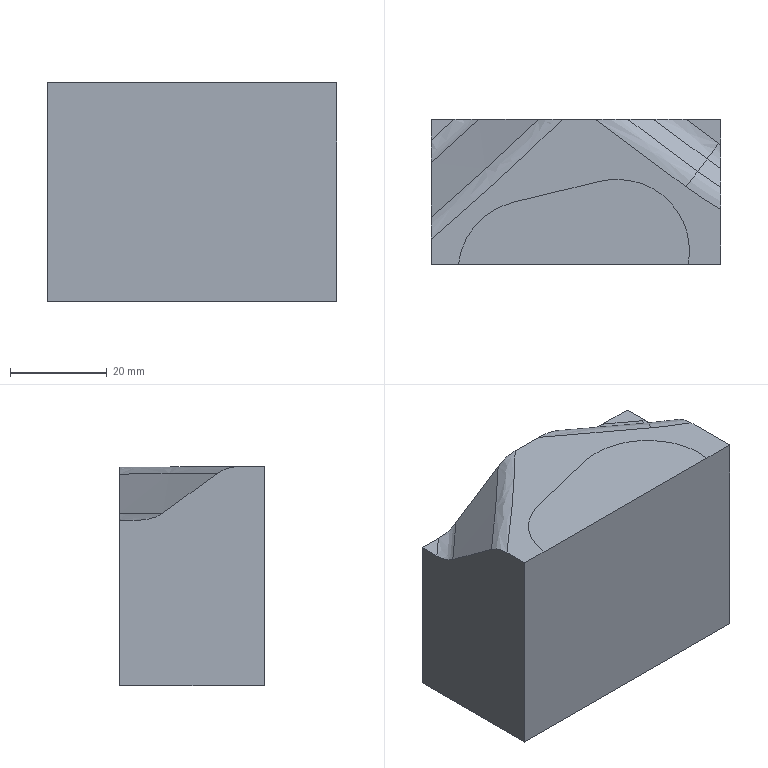Part | NX | features solid 2 | 1 solid | 18 faces | box 60 x 30 x 45.393 mm | volume 79393 mm3 | spline 13 | plane 5
STEP:
#1=CARTESIAN_POINT('',(-430.,-95.,60.393));
#2=VERTEX_POINT('',#1);
#3=CARTESIAN_POINT('',(-424.352,-95.,60.385));
#4=VERTEX_POINT('',#3);
#5=CARTESIAN_POINT('',(-429.926,-95.,60.393));
#6=DIRECTION('',(1.,0.,-0.001477));
#7=VECTOR('',#6,1000.);
#8=LINE('',#5,#7);
#9=EDGE_CURVE('',#2,#4,#8,.T.);
#10=ORIENTED_EDGE('',*,*,#9,.F.);
#11=CARTESIAN_POINT('',(-430.,-95.,15.));
#12=VERTEX_POINT('',#11);
#13=CARTESIAN_POINT('',(-430.,-95.,10.));
#14=DIRECTION('',(0.,0.,1.));
#15=VECTOR('',#14,1000.);
#16=LINE('',#13,#15);
#17=EDGE_CURVE('',#12,#2,#16,.T.);
#18=ORIENTED_EDGE('',*,*,#17,.F.);
#19=CARTESIAN_POINT('',(-370.,-95.,15.));
#20=VERTEX_POINT('',#19);
#21=CARTESIAN_POINT('',(-430.,-95.,15.));
#22=DIRECTION('',(1.,0.,0.));
#23=VECTOR('',#22,1000.);
#24=LINE('',#21,#23);
#25=EDGE_CURVE('',#12,#20,#24,.T.);
#26=ORIENTED_EDGE('',*,*,#25,.T.);
#27=CARTESIAN_POINT('',(-370.,-95.,60.305));
#28=VERTEX_POINT('',#27);
#29=CARTESIAN_POINT('',(-370.,-95.,10.));
#30=DIRECTION('',(0.,0.,1.));
#31=VECTOR('',#30,1000.);
#32=LINE('',#29,#31);
#33=EDGE_CURVE('',#20,#28,#32,.T.);
#34=ORIENTED_EDGE('',*,*,#33,.T.);
#35=CARTESIAN_POINT('',(-376.703,-95.,60.314));
#36=VERTEX_POINT('',#35);
#37=CARTESIAN_POINT('',(-429.926,-95.,60.393));
#38=DIRECTION('',(1.,0.,-0.001477));
#39=VECTOR('',#38,1000.);
#40=LINE('',#37,#39);
#41=EDGE_CURVE('',#36,#28,#40,.T.);
#42=ORIENTED_EDGE('',*,*,#41,.F.);
#43=CARTESIAN_POINT('',(-429.926,-95.,60.393));
#44=DIRECTION('',(1.,0.,-0.001477));
#45=VECTOR('',#44,1000.);
#46=LINE('',#43,#45);
#47=EDGE_CURVE('',#4,#36,#46,.T.);
#48=ORIENTED_EDGE('',*,*,#47,.F.);
#49=EDGE_LOOP('',(#10,#18,#26,#34,#42,#48));
#50=FACE_BOUND('',#49,.T.);
#51=CARTESIAN_POINT('',(-430.,-95.,10.));
#52=DIRECTION('',(0.,-1.,0.));
#53=DIRECTION('',(0.,0.,1.));
#54=AXIS2_PLACEMENT_3D('',#51,#52,#53);
#55=PLANE('',#54);
#56=ADVANCED_FACE('',(#50),#55,.T.);
#57=CARTESIAN_POINT('',(-425.27,-65.,49.259));
#58=VERTEX_POINT('',#57);
#59=CARTESIAN_POINT('',(-430.,-65.,49.276));
#60=VERTEX_POINT('',#59);
#61=CARTESIAN_POINT('',(-429.855,-65.,49.276));
#62=DIRECTION('',(1.,0.,-0.003698));
#63=VECTOR('',#62,1000.);
#64=LINE('',#61,#63);
#65=EDGE_CURVE('',#58,#60,#64,.F.);
#66=ORIENTED_EDGE('',*,*,#65,.F.);
#67=CARTESIAN_POINT('',(-420.138,-65.,50.648));
#68=VERTEX_POINT('',#67);
#69=CARTESIAN_POINT('',(-425.274,-65.,49.259));
#70=CARTESIAN_POINT('',(-423.471,-65.,49.252));
#71=CARTESIAN_POINT('',(-421.65,-65.,49.659));
#72=CARTESIAN_POINT('',(-420.138,-65.,50.648));
#73=B_SPLINE_CURVE_WITH_KNOTS('',3,(#69,#70,#71,#72),.UNSPECIFIED.,.F.,.F.,(4,4),(0.,0.005391),.UNSPECIFIED.);
#74=EDGE_CURVE('',#58,#68,#73,.T.);
#75=ORIENTED_EDGE('',*,*,#74,.T.);
#76=CARTESIAN_POINT('',(-407.783,-65.,58.79));
#77=VERTEX_POINT('',#76);
#78=CARTESIAN_POINT('',(-407.783,-65.,58.79));
#79=CARTESIAN_POINT('',(-411.892,-65.,56.061));
#80=CARTESIAN_POINT('',(-416.01,-65.,53.346));
#81=CARTESIAN_POINT('',(-420.138,-65.,50.648));
#82=B_SPLINE_CURVE_WITH_KNOTS('',3,(#78,#79,#80,#81),.UNSPECIFIED.,.F.,.F.,(4,4),(0.00008889,0.01488),.UNSPECIFIED.);
#83=EDGE_CURVE('',#77,#68,#82,.T.);
#84=ORIENTED_EDGE('',*,*,#83,.F.);
#85=CARTESIAN_POINT('',(-402.801,-65.,60.174));
#86=VERTEX_POINT('',#85);
#87=CARTESIAN_POINT('',(-407.783,-65.,58.79));
#88=CARTESIAN_POINT('',(-406.319,-65.,59.762));
#89=CARTESIAN_POINT('',(-404.555,-65.,60.177));
#90=CARTESIAN_POINT('',(-402.801,-65.,60.174));
#91=B_SPLINE_CURVE_WITH_KNOTS('',3,(#87,#88,#89,#90),.UNSPECIFIED.,.F.,.F.,(4,4),(0.,0.005252),.UNSPECIFIED.);
#92=EDGE_CURVE('',#77,#86,#91,.T.);
#93=ORIENTED_EDGE('',*,*,#92,.T.);
#94=CARTESIAN_POINT('',(-395.934,-65.,60.164));
#95=VERTEX_POINT('',#94);
#96=CARTESIAN_POINT('',(-429.926,-65.,60.214));
#97=DIRECTION('',(1.,0.,-0.001477));
#98=VECTOR('',#97,1000.);
#99=LINE('',#96,#98);
#100=EDGE_CURVE('',#95,#86,#99,.F.);
#101=ORIENTED_EDGE('',*,*,#100,.F.);
#102=CARTESIAN_POINT('',(-389.261,-65.,58.622));
#103=VERTEX_POINT('',#102);
#104=CARTESIAN_POINT('',(-395.934,-65.,60.164));
#105=CARTESIAN_POINT('',(-393.624,-65.,60.161));
#106=CARTESIAN_POINT('',(-391.295,-65.,59.722));
#107=CARTESIAN_POINT('',(-389.261,-65.,58.622));
#108=B_SPLINE_CURVE_WITH_KNOTS('',3,(#104,#105,#106,#107),.UNSPECIFIED.,.F.,.F.,(4,4),(0.,0.006914),.UNSPECIFIED.);
#109=EDGE_CURVE('',#95,#103,#108,.T.);
#110=ORIENTED_EDGE('',*,*,#109,.T.);
#111=CARTESIAN_POINT('',(-383.886,-65.,55.715));
#112=VERTEX_POINT('',#111);
#113=CARTESIAN_POINT('',(-400.43,-65.,64.664));
#114=DIRECTION('',(-0.8796,0.,0.4758));
#115=VECTOR('',#114,1000.);
#116=LINE('',#113,#115);
#117=EDGE_CURVE('',#103,#112,#116,.F.);
#118=ORIENTED_EDGE('',*,*,#117,.T.);
#119=CARTESIAN_POINT('',(-377.192,-65.,54.164));
#120=VERTEX_POINT('',#119);
#121=CARTESIAN_POINT('',(-377.192,-65.,54.164));
#122=CARTESIAN_POINT('',(-379.509,-65.,54.17));
#123=CARTESIAN_POINT('',(-381.845,-65.,54.611));
#124=CARTESIAN_POINT('',(-383.886,-65.,55.715));
#125=B_SPLINE_CURVE_WITH_KNOTS('',3,(#121,#122,#123,#124),.UNSPECIFIED.,.F.,.F.,(4,4),(0.000043,0.00698),.UNSPECIFIED.);
#126=EDGE_CURVE('',#120,#112,#125,.T.);
#127=ORIENTED_EDGE('',*,*,#126,.F.);
#128=CARTESIAN_POINT('',(-370.,-65.,54.145));
#129=VERTEX_POINT('',#128);
#130=CARTESIAN_POINT('',(-429.886,-65.,54.3));
#131=DIRECTION('',(1.,0.,-0.002576));
#132=VECTOR('',#131,1000.);
#133=LINE('',#130,#132);
#134=EDGE_CURVE('',#129,#120,#133,.F.);
#135=ORIENTED_EDGE('',*,*,#134,.F.);
#136=CARTESIAN_POINT('',(-370.,-65.,15.));
#137=VERTEX_POINT('',#136);
#138=CARTESIAN_POINT('',(-370.,-65.,10.));
#139=DIRECTION('',(0.,0.,1.));
#140=VECTOR('',#139,1000.);
#141=LINE('',#138,#140);
#142=EDGE_CURVE('',#137,#129,#141,.T.);
#143=ORIENTED_EDGE('',*,*,#142,.F.);
#144=CARTESIAN_POINT('',(-430.,-65.,15.));
#145=VERTEX_POINT('',#144);
#146=CARTESIAN_POINT('',(-430.,-65.,15.));
#147=DIRECTION('',(-1.,0.,0.));
#148=VECTOR('',#147,1000.);
#149=LINE('',#146,#148);
#150=EDGE_CURVE('',#145,#137,#149,.F.);
#151=ORIENTED_EDGE('',*,*,#150,.F.);
#152=CARTESIAN_POINT('',(-430.,-65.,10.));
#153=DIRECTION('',(0.,0.,1.));
#154=VECTOR('',#153,1000.);
#155=LINE('',#152,#154);
#156=EDGE_CURVE('',#145,#60,#155,.T.);
#157=ORIENTED_EDGE('',*,*,#156,.T.);
#158=EDGE_LOOP('',(#66,#75,#84,#93,#101,#110,#118,#127,#135,#143,#151,#157));
#159=FACE_BOUND('',#158,.T.);
#160=CARTESIAN_POINT('',(-430.,-65.,10.));
#161=DIRECTION('',(0.,-1.,0.));
#162=DIRECTION('',(0.,0.,1.));
#163=AXIS2_PLACEMENT_3D('',#160,#161,#162);
#164=PLANE('',#163);
#165=ADVANCED_FACE('',(#159),#164,.F.);
#166=CARTESIAN_POINT('',(-370.,-83.647,60.237));
#167=VERTEX_POINT('',#166);
#168=CARTESIAN_POINT('',(-370.,-64.701,60.124));
#169=DIRECTION('',(0.,-1.,0.005958));
#170=VECTOR('',#169,1000.);
#171=LINE('',#168,#170);
#172=EDGE_CURVE('',#28,#167,#171,.F.);
#173=ORIENTED_EDGE('',*,*,#172,.F.);
#174=ORIENTED_EDGE('',*,*,#33,.F.);
#175=CARTESIAN_POINT('',(-370.,-65.,15.));
#176=DIRECTION('',(0.,1.,0.));
#177=VECTOR('',#176,1000.);
#178=LINE('',#175,#177);
#179=EDGE_CURVE('',#137,#20,#178,.F.);
#180=ORIENTED_EDGE('',*,*,#179,.F.);
#181=ORIENTED_EDGE('',*,*,#142,.T.);
#182=CARTESIAN_POINT('',(-370.,-70.351,54.17));
#183=VERTEX_POINT('',#182);
#184=CARTESIAN_POINT('',(-370.,-64.798,54.145));
#185=DIRECTION('',(0.,-1.,0.004576));
#186=VECTOR('',#185,1000.);
#187=LINE('',#184,#186);
#188=EDGE_CURVE('',#183,#129,#187,.F.);
#189=ORIENTED_EDGE('',*,*,#188,.F.);
#190=CARTESIAN_POINT('',(-370.,-75.202,55.727));
#191=VERTEX_POINT('',#190);
#192=CARTESIAN_POINT('',(-370.,-75.202,55.726));
#193=CARTESIAN_POINT('',(-370.,-73.815,54.672));
#194=CARTESIAN_POINT('',(-370.,-72.09,54.178));
#195=CARTESIAN_POINT('',(-370.,-70.351,54.17));
#196=B_SPLINE_CURVE_WITH_KNOTS('',3,(#192,#193,#194,#195),.UNSPECIFIED.,.F.,.F.,(4,4),(0.,0.005159),.UNSPECIFIED.);
#197=EDGE_CURVE('',#191,#183,#196,.T.);
#198=ORIENTED_EDGE('',*,*,#197,.F.);
#199=CARTESIAN_POINT('',(-370.,-79.036,58.677));
#200=VERTEX_POINT('',#199);
#201=CARTESIAN_POINT('',(-370.,-75.203,55.727));
#202=CARTESIAN_POINT('',(-370.,-76.486,56.703));
#203=CARTESIAN_POINT('',(-370.,-77.764,57.687));
#204=CARTESIAN_POINT('',(-370.,-79.036,58.677));
#205=B_SPLINE_CURVE_WITH_KNOTS('',3,(#201,#202,#203,#204),.UNSPECIFIED.,.F.,.F.,(4,4),(0.00008367,0.004921),.UNSPECIFIED.);
#206=EDGE_CURVE('',#191,#200,#205,.T.);
#207=ORIENTED_EDGE('',*,*,#206,.T.);
#208=CARTESIAN_POINT('',(-370.,-83.646,60.237));
#209=CARTESIAN_POINT('',(-370.,-81.988,60.227));
#210=CARTESIAN_POINT('',(-370.,-80.346,59.696));
#211=CARTESIAN_POINT('',(-370.,-79.036,58.677));
#212=B_SPLINE_CURVE_WITH_KNOTS('',3,(#208,#209,#210,#211),.UNSPECIFIED.,.F.,.F.,(4,4),(0.,0.004923),.UNSPECIFIED.);
#213=EDGE_CURVE('',#167,#200,#212,.T.);
#214=ORIENTED_EDGE('',*,*,#213,.F.);
#215=EDGE_LOOP('',(#173,#174,#180,#181,#189,#198,#207,#214));
#216=FACE_BOUND('',#215,.T.);
#217=CARTESIAN_POINT('',(-370.,-65.,10.));
#218=DIRECTION('',(-1.,0.,0.));
#219=DIRECTION('',(0.,0.,1.));
#220=AXIS2_PLACEMENT_3D('',#217,#218,#219);
#221=PLANE('',#220);
#222=ADVANCED_FACE('',(#216),#221,.F.);
#223=CARTESIAN_POINT('',(-430.,-69.285,49.284));
#224=VERTEX_POINT('',#223);
#225=CARTESIAN_POINT('',(-430.,-73.938,50.7));
#226=VERTEX_POINT('',#225);
#227=CARTESIAN_POINT('',(-430.,-69.278,49.284));
#228=CARTESIAN_POINT('',(-430.,-70.934,49.287));
#229=CARTESIAN_POINT('',(-430.,-72.595,49.725));
#230=CARTESIAN_POINT('',(-430.,-73.938,50.7));
#231=B_SPLINE_CURVE_WITH_KNOTS('',3,(#227,#228,#229,#230),.UNSPECIFIED.,.F.,.F.,(4,4),(0.,0.004952),.UNSPECIFIED.);
#232=EDGE_CURVE('',#224,#226,#231,.T.);
#233=ORIENTED_EDGE('',*,*,#232,.F.);
#234=CARTESIAN_POINT('',(-430.,-64.931,49.276));
#235=DIRECTION('',(0.,-1.,0.00175));
#236=VECTOR('',#235,1000.);
#237=LINE('',#234,#236);
#238=EDGE_CURVE('',#224,#60,#237,.F.);
#239=ORIENTED_EDGE('',*,*,#238,.T.);
#240=ORIENTED_EDGE('',*,*,#156,.F.);
#241=CARTESIAN_POINT('',(-430.,-65.,15.));
#242=DIRECTION('',(0.,1.,0.));
#243=VECTOR('',#242,1000.);
#244=LINE('',#241,#243);
#245=EDGE_CURVE('',#145,#12,#244,.F.);
#246=ORIENTED_EDGE('',*,*,#245,.T.);
#247=ORIENTED_EDGE('',*,*,#17,.T.);
#248=CARTESIAN_POINT('',(-430.,-89.798,60.362));
#249=VERTEX_POINT('',#248);
#250=CARTESIAN_POINT('',(-430.,-64.701,60.213));
#251=DIRECTION('',(0.,-1.,0.005958));
#252=VECTOR('',#251,1000.);
#253=LINE('',#250,#252);
#254=EDGE_CURVE('',#2,#249,#253,.F.);
#255=ORIENTED_EDGE('',*,*,#254,.T.);
#256=CARTESIAN_POINT('',(-430.,-85.235,58.943));
#257=VERTEX_POINT('',#256);
#258=CARTESIAN_POINT('',(-430.,-85.235,58.943));
#259=CARTESIAN_POINT('',(-430.,-86.549,59.908));
#260=CARTESIAN_POINT('',(-430.,-88.17,60.352));
#261=CARTESIAN_POINT('',(-430.,-89.797,60.362));
#262=B_SPLINE_CURVE_WITH_KNOTS('',3,(#258,#259,#260,#261),.UNSPECIFIED.,.F.,.F.,(4,4),(0.,0.004839),.UNSPECIFIED.);
#263=EDGE_CURVE('',#257,#249,#262,.T.);
#264=ORIENTED_EDGE('',*,*,#263,.F.);
#265=CARTESIAN_POINT('',(-430.,-85.235,58.943));
#266=CARTESIAN_POINT('',(-430.,-81.476,56.185));
#267=CARTESIAN_POINT('',(-430.,-77.711,53.438));
#268=CARTESIAN_POINT('',(-430.,-73.938,50.7));
#269=B_SPLINE_CURVE_WITH_KNOTS('',3,(#265,#266,#267,#268),.UNSPECIFIED.,.F.,.F.,(4,4),(0.000084,0.01407),.UNSPECIFIED.);
#270=EDGE_CURVE('',#257,#226,#269,.T.);
#271=ORIENTED_EDGE('',*,*,#270,.T.);
#272=EDGE_LOOP('',(#233,#239,#240,#246,#247,#255,#264,#271));
#273=FACE_BOUND('',#272,.T.);
#274=CARTESIAN_POINT('',(-430.,-65.,10.));
#275=DIRECTION('',(-1.,0.,0.));
#276=DIRECTION('',(0.,0.,1.));
#277=AXIS2_PLACEMENT_3D('',#274,#275,#276);
#278=PLANE('',#277);
#279=ADVANCED_FACE('',(#273),#278,.T.);
#280=ORIENTED_EDGE('',*,*,#150,.T.);
#281=ORIENTED_EDGE('',*,*,#179,.T.);
#282=ORIENTED_EDGE('',*,*,#25,.F.);
#283=ORIENTED_EDGE('',*,*,#245,.F.);
#284=EDGE_LOOP('',(#280,#281,#282,#283));
#285=FACE_BOUND('',#284,.T.);
#286=CARTESIAN_POINT('',(-430.,-65.,15.));
#287=DIRECTION('',(0.,0.,-1.));
#288=DIRECTION('',(0.,-1.,0.));
#289=AXIS2_PLACEMENT_3D('',#286,#287,#288);
#290=PLANE('',#289);
#291=ADVANCED_FACE('',(#285),#290,.T.);
#292=ORIENTED_EDGE('',*,*,#47,.T.);
#293=CARTESIAN_POINT('',(-394.978,-77.819,60.239));
#294=VERTEX_POINT('',#293);
#295=CARTESIAN_POINT('',(-376.705,-94.999,60.314));
#296=CARTESIAN_POINT('',(-376.275,-92.541,60.299));
#297=CARTESIAN_POINT('',(-376.637,-87.429,60.269));
#298=CARTESIAN_POINT('',(-380.148,-82.049,60.242));
#299=CARTESIAN_POINT('',(-384.224,-79.074,60.231));
#300=CARTESIAN_POINT('',(-387.107,-77.972,60.228));
#301=CARTESIAN_POINT('',(-389.571,-77.528,60.229));
#302=CARTESIAN_POINT('',(-391.094,-77.444,60.231));
#303=CARTESIAN_POINT('',(-392.189,-77.471,60.233));
#304=CARTESIAN_POINT('',(-392.865,-77.517,60.234));
#305=CARTESIAN_POINT('',(-393.655,-77.591,60.236));
#306=CARTESIAN_POINT('',(-394.358,-77.698,60.237));
#307=CARTESIAN_POINT('',(-394.979,-77.816,60.239));
#308=B_SPLINE_CURVE_WITH_KNOTS('',3,(#295,#296,#297,#298,#299,#300,#301,#302,#303,#304,#305,#306,#307),.UNSPECIFIED.,.F.,.F.,(4,1,1,1,1,1,1,1,1,1,4),(0.6328,0.6897,0.7467,0.7751,0.8036,0.8178,0.8321,0.8392,0.8427,0.8463,0.8605),.UNSPECIFIED.);
#309=EDGE_CURVE('',#36,#294,#308,.T.);
#310=ORIENTED_EDGE('',*,*,#309,.T.);
#311=CARTESIAN_POINT('',(-412.965,-82.147,60.291));
#312=VERTEX_POINT('',#311);
#313=CARTESIAN_POINT('',(-394.979,-77.816,60.239));
#314=CARTESIAN_POINT('',(-395.358,-77.888,60.24));
#315=CARTESIAN_POINT('',(-395.944,-78.012,60.242));
#316=CARTESIAN_POINT('',(-396.713,-78.195,60.244));
#317=CARTESIAN_POINT('',(-397.111,-78.296,60.245));
#318=CARTESIAN_POINT('',(-397.49,-78.391,60.246));
#319=CARTESIAN_POINT('',(-398.186,-78.566,60.248));
#320=CARTESIAN_POINT('',(-399.446,-78.879,60.252));
#321=CARTESIAN_POINT('',(-401.216,-79.314,60.257));
#322=CARTESIAN_POINT('',(-403.217,-79.801,60.263));
#323=CARTESIAN_POINT('',(-404.724,-80.165,60.267));
#324=CARTESIAN_POINT('',(-405.531,-80.36,60.27));
#325=CARTESIAN_POINT('',(-405.963,-80.464,60.271));
#326=CARTESIAN_POINT('',(-406.545,-80.604,60.273));
#327=CARTESIAN_POINT('',(-407.327,-80.792,60.275));
#328=CARTESIAN_POINT('',(-408.437,-81.059,60.278));
#329=CARTESIAN_POINT('',(-410.177,-81.477,60.283));
#330=CARTESIAN_POINT('',(-411.996,-81.914,60.289));
#331=CARTESIAN_POINT('',(-412.758,-82.098,60.291));
#332=CARTESIAN_POINT('',(-412.965,-82.147,60.291));
#333=B_SPLINE_CURVE_WITH_KNOTS('',3,(#313,#314,#315,#316,#317,#318,#319,#320,#321,#322,#323,#324,#325,#326,#327,#328,#329,#330,#331,#332),.UNSPECIFIED.,.F.,.F.,(4,1,1,1,1,1,1,1,1,1,1,1,1,1,1,1,1,4),(0.8605,0.8693,0.8736,0.8758,0.878,0.8867,0.8954,0.9128,0.9303,0.939,0.9433,0.9455,0.9477,0.9521,0.9564,0.9651,0.9826,1.),.UNSPECIFIED.);
#334=EDGE_CURVE('',#294,#312,#333,.T.);
#335=ORIENTED_EDGE('',*,*,#334,.T.);
#336=CARTESIAN_POINT('',(-412.965,-82.147,60.291));
#337=CARTESIAN_POINT('',(-415.91,-82.856,60.3));
#338=CARTESIAN_POINT('',(-420.051,-85.39,60.321));
#339=CARTESIAN_POINT('',(-423.351,-90.457,60.356));
#340=CARTESIAN_POINT('',(-424.171,-93.491,60.376));
#341=CARTESIAN_POINT('',(-424.35,-95.,60.385));
#342=B_SPLINE_CURVE_WITH_KNOTS('',3,(#336,#337,#338,#339,#340,#341),.UNSPECIFIED.,.F.,.F.,(4,1,1,4),(0.,0.06962,0.1044,0.1392),.UNSPECIFIED.);
#343=EDGE_CURVE('',#312,#4,#342,.T.);
#344=ORIENTED_EDGE('',*,*,#343,.T.);
#345=EDGE_LOOP('',(#292,#310,#335,#344));
#346=FACE_BOUND('',#345,.T.);
#347=CARTESIAN_POINT('',(-424.637,-95.106,60.386));
#348=CARTESIAN_POINT('',(-376.173,-95.106,60.314));
#349=CARTESIAN_POINT('',(-424.637,-77.33,60.28));
#350=CARTESIAN_POINT('',(-376.173,-77.33,60.208));
#351=B_SPLINE_SURFACE_WITH_KNOTS('',1,1,((#347,#348),(#349,#350)),.PLANE_SURF.,.F.,.F.,.F.,(2,2),(2,2),(0.7159,0.8657),(0.2377,0.4034),.PIECEWISE_BEZIER_KNOTS.);
#352=ADVANCED_FACE('',(#346),#351,.F.);
#353=CARTESIAN_POINT('',(-377.227,-78.986,60.22));
#354=VERTEX_POINT('',#353);
#355=CARTESIAN_POINT('',(-377.227,-78.986,60.22));
#356=CARTESIAN_POINT('',(-383.463,-74.324,60.201));
#357=CARTESIAN_POINT('',(-389.698,-69.662,60.183));
#358=CARTESIAN_POINT('',(-395.934,-65.,60.164));
#359=B_SPLINE_CURVE_WITH_KNOTS('',3,(#355,#356,#357,#358),.UNSPECIFIED.,.F.,.F.,(4,4),(0.,0.8279),.UNSPECIFIED.);
#360=EDGE_CURVE('',#95,#354,#359,.F.);
#361=ORIENTED_EDGE('',*,*,#360,.T.);
#362=CARTESIAN_POINT('',(-374.832,-75.788,58.665));
#363=VERTEX_POINT('',#362);
#364=CARTESIAN_POINT('',(-374.832,-75.788,58.665));
#365=CARTESIAN_POINT('',(-375.468,-76.635,59.625));
#366=CARTESIAN_POINT('',(-376.372,-77.842,60.212));
#367=CARTESIAN_POINT('',(-377.227,-78.986,60.22));
#368=B_SPLINE_CURVE_WITH_KNOTS('',3,(#364,#365,#366,#367),.UNSPECIFIED.,.F.,.F.,(4,4),(0.,1.),.UNSPECIFIED.);
#369=EDGE_CURVE('',#354,#363,#368,.F.);
#370=ORIENTED_EDGE('',*,*,#369,.T.);
#371=CARTESIAN_POINT('',(-389.261,-65.,58.622));
#372=CARTESIAN_POINT('',(-384.451,-68.596,58.637));
#373=CARTESIAN_POINT('',(-379.641,-72.192,58.651));
#374=CARTESIAN_POINT('',(-374.832,-75.788,58.665));
#375=B_SPLINE_CURVE_WITH_KNOTS('',3,(#371,#372,#373,#374),.UNSPECIFIED.,.F.,.F.,(4,4),(0.3652,1.),.UNSPECIFIED.);
#376=EDGE_CURVE('',#103,#363,#375,.T.);
#377=ORIENTED_EDGE('',*,*,#376,.F.);
#378=ORIENTED_EDGE('',*,*,#109,.F.);
#379=EDGE_LOOP('',(#361,#370,#377,#378));
#380=FACE_BOUND('',#379,.T.);
#381=CARTESIAN_POINT('',(-374.832,-75.788,58.665));
#382=CARTESIAN_POINT('',(-393.65,-61.718,58.609));
#383=CARTESIAN_POINT('',(-375.497,-76.674,59.669));
#384=CARTESIAN_POINT('',(-394.315,-62.604,59.613));
#385=CARTESIAN_POINT('',(-376.332,-77.789,60.211));
#386=CARTESIAN_POINT('',(-395.151,-63.719,60.155));
#387=CARTESIAN_POINT('',(-377.227,-78.986,60.22));
#388=CARTESIAN_POINT('',(-396.046,-64.916,60.164));
#389=(BOUNDED_SURFACE()B_SPLINE_SURFACE(3,1,((#381,#382),(#383,#384),(#385,#386),(#387,#388)),.CYLINDRICAL_SURF.,.F.,.F.,.F.)B_SPLINE_SURFACE_WITH_KNOTS((4,4),(2,2),(0.006098,1.),(0.,0.823),.PIECEWISE_BEZIER_KNOTS.)GEOMETRIC_REPRESENTATION_ITEM()RATIONAL_B_SPLINE_SURFACE(((0.9992,0.9992),(0.9555,0.9555),(0.9557,0.9557),(1.,1.)))REPRESENTATION_ITEM('')SURFACE());
#390=ADVANCED_FACE('',(#380),#389,.F.);
#391=ORIENTED_EDGE('',*,*,#376,.T.);
#392=CARTESIAN_POINT('',(-372.883,-73.194,55.724));
#393=VERTEX_POINT('',#392);
#394=CARTESIAN_POINT('',(-374.832,-75.788,58.665));
#395=CARTESIAN_POINT('',(-374.182,-74.924,57.685));
#396=CARTESIAN_POINT('',(-373.533,-74.059,56.705));
#397=CARTESIAN_POINT('',(-372.883,-73.194,55.724));
#398=B_SPLINE_CURVE_WITH_KNOTS('',3,(#394,#395,#396,#397),.UNSPECIFIED.,.F.,.F.,(4,4),(0.,1.),.UNSPECIFIED.);
#399=EDGE_CURVE('',#363,#393,#398,.T.);
#400=ORIENTED_EDGE('',*,*,#399,.T.);
#401=CARTESIAN_POINT('',(-372.883,-73.194,55.724));
#402=CARTESIAN_POINT('',(-376.551,-70.463,55.721));
#403=CARTESIAN_POINT('',(-380.219,-67.731,55.718));
#404=CARTESIAN_POINT('',(-383.886,-65.,55.715));
#405=B_SPLINE_CURVE_WITH_KNOTS('',3,(#401,#402,#403,#404),.UNSPECIFIED.,.F.,.F.,(4,4),(0.,0.4436),.UNSPECIFIED.);
#406=EDGE_CURVE('',#393,#112,#405,.T.);
#407=ORIENTED_EDGE('',*,*,#406,.T.);
#408=ORIENTED_EDGE('',*,*,#117,.F.);
#409=EDGE_LOOP('',(#391,#400,#407,#408));
#410=FACE_BOUND('',#409,.T.);
#411=CARTESIAN_POINT('',(-389.359,-63.541,57.614));
#412=CARTESIAN_POINT('',(-372.785,-67.806,51.751));
#413=CARTESIAN_POINT('',(-389.359,-72.101,63.841));
#414=CARTESIAN_POINT('',(-372.785,-76.366,57.978));
#415=B_SPLINE_SURFACE_WITH_KNOTS('',1,1,((#411,#412),(#413,#414)),.PLANE_SURF.,.F.,.F.,.F.,(2,2),(2,2),(0.4403,0.9974),(0.3377,0.998),.PIECEWISE_BEZIER_KNOTS.);
#416=ADVANCED_FACE('',(#410),#415,.T.);
#417=ORIENTED_EDGE('',*,*,#126,.T.);
#418=ORIENTED_EDGE('',*,*,#406,.F.);
#419=CARTESIAN_POINT('',(-370.494,-69.988,54.17));
#420=VERTEX_POINT('',#419);
#421=CARTESIAN_POINT('',(-372.883,-73.194,55.724));
#422=CARTESIAN_POINT('',(-372.25,-72.345,54.764));
#423=CARTESIAN_POINT('',(-371.349,-71.135,54.177));
#424=CARTESIAN_POINT('',(-370.494,-69.988,54.17));
#425=B_SPLINE_CURVE_WITH_KNOTS('',3,(#421,#422,#423,#424),.UNSPECIFIED.,.F.,.F.,(4,4),(0.,1.),.UNSPECIFIED.);
#426=EDGE_CURVE('',#393,#420,#425,.T.);
#427=ORIENTED_EDGE('',*,*,#426,.T.);
#428=CARTESIAN_POINT('',(-370.494,-69.988,54.17));
#429=CARTESIAN_POINT('',(-372.727,-68.325,54.168));
#430=CARTESIAN_POINT('',(-374.959,-66.663,54.166));
#431=CARTESIAN_POINT('',(-377.192,-65.,54.164));
#432=B_SPLINE_CURVE_WITH_KNOTS('',3,(#428,#429,#430,#431),.UNSPECIFIED.,.F.,.F.,(4,4),(0.,0.2545),.UNSPECIFIED.);
#433=EDGE_CURVE('',#420,#120,#432,.T.);
#434=ORIENTED_EDGE('',*,*,#433,.T.);
#435=EDGE_LOOP('',(#417,#418,#427,#434));
#436=FACE_BOUND('',#435,.T.);
#437=CARTESIAN_POINT('',(-372.883,-73.194,55.724));
#438=CARTESIAN_POINT('',(-383.952,-64.951,55.715));
#439=CARTESIAN_POINT('',(-372.221,-72.306,54.72));
#440=CARTESIAN_POINT('',(-383.29,-64.062,54.71));
#441=CARTESIAN_POINT('',(-371.388,-71.188,54.177));
#442=CARTESIAN_POINT('',(-382.457,-62.944,54.168));
#443=CARTESIAN_POINT('',(-370.494,-69.988,54.17));
#444=CARTESIAN_POINT('',(-381.563,-61.744,54.16));
#445=(BOUNDED_SURFACE()B_SPLINE_SURFACE(3,1,((#437,#438),(#439,#440),(#441,#442),(#443,#444)),.CYLINDRICAL_SURF.,.F.,.F.,.F.)B_SPLINE_SURFACE_WITH_KNOTS((4,4),(2,2),(0.,0.9939),(0.,0.4146),.PIECEWISE_BEZIER_KNOTS.)GEOMETRIC_REPRESENTATION_ITEM()RATIONAL_B_SPLINE_SURFACE(((1.,1.),(0.9557,0.9557),(0.9554,0.9554),(0.9992,0.9992)))REPRESENTATION_ITEM('')SURFACE());
#446=ADVANCED_FACE('',(#436),#445,.T.);
#447=ORIENTED_EDGE('',*,*,#213,.T.);
#448=CARTESIAN_POINT('',(-374.832,-75.788,58.665));
#449=CARTESIAN_POINT('',(-373.285,-76.945,58.67));
#450=CARTESIAN_POINT('',(-371.671,-78.031,58.674));
#451=CARTESIAN_POINT('',(-370.,-79.036,58.677));
#452=B_SPLINE_CURVE_WITH_KNOTS('',3,(#448,#449,#450,#451),.UNSPECIFIED.,.F.,.F.,(4,4),(0.,0.2094),.UNSPECIFIED.);
#453=EDGE_CURVE('',#363,#200,#452,.T.);
#454=ORIENTED_EDGE('',*,*,#453,.F.);
#455=ORIENTED_EDGE('',*,*,#369,.F.);
#456=CARTESIAN_POINT('',(-370.,-83.647,60.237));
#457=CARTESIAN_POINT('',(-372.526,-82.256,60.232));
#458=CARTESIAN_POINT('',(-374.945,-80.693,60.227));
#459=CARTESIAN_POINT('',(-377.227,-78.986,60.22));
#460=B_SPLINE_CURVE_WITH_KNOTS('',3,(#456,#457,#458,#459),.UNSPECIFIED.,.F.,.F.,(4,4),(0.7109,1.),.UNSPECIFIED.);
#461=EDGE_CURVE('',#354,#167,#460,.F.);
#462=ORIENTED_EDGE('',*,*,#461,.T.);
#463=EDGE_LOOP('',(#447,#454,#455,#462));
#464=FACE_BOUND('',#463,.T.);
#465=CARTESIAN_POINT('',(-368.028,-80.171,58.681));
#466=CARTESIAN_POINT('',(-370.4,-78.867,58.677));
#467=CARTESIAN_POINT('',(-372.672,-77.403,58.672));
#468=CARTESIAN_POINT('',(-374.832,-75.788,58.665));
#469=CARTESIAN_POINT('',(-368.562,-81.141,59.686));
#470=CARTESIAN_POINT('',(-370.981,-79.812,59.681));
#471=CARTESIAN_POINT('',(-373.295,-78.32,59.676));
#472=CARTESIAN_POINT('',(-375.497,-76.674,59.669));
#473=CARTESIAN_POINT('',(-369.234,-82.362,60.228));
#474=CARTESIAN_POINT('',(-371.709,-81.001,60.224));
#475=CARTESIAN_POINT('',(-374.079,-79.474,60.218));
#476=CARTESIAN_POINT('',(-376.332,-77.789,60.211));
#477=CARTESIAN_POINT('',(-369.954,-83.672,60.237));
#478=CARTESIAN_POINT('',(-372.491,-82.278,60.232));
#479=CARTESIAN_POINT('',(-374.919,-80.713,60.227));
#480=CARTESIAN_POINT('',(-377.227,-78.986,60.22));
#481=(BOUNDED_SURFACE()B_SPLINE_SURFACE(3,3,((#465,#466,#467,#468),(#469,#470,#471,#472),(#473,#474,#475,#476),(#477,#478,#479,#480)),.TOROIDAL_SURF.,.F.,.F.,.F.)B_SPLINE_SURFACE_WITH_KNOTS((4,4),(4,4),(0.,1.),(0.7092,1.),.PIECEWISE_BEZIER_KNOTS.)GEOMETRIC_REPRESENTATION_ITEM()RATIONAL_B_SPLINE_SURFACE(((0.9881,0.9905,0.9944,1.),(0.9446,0.9469,0.9507,0.956),(0.9446,0.9469,0.9507,0.956),(0.9881,0.9905,0.9944,1.)))REPRESENTATION_ITEM('')SURFACE());
#482=ADVANCED_FACE('',(#464),#481,.F.);
#483=ORIENTED_EDGE('',*,*,#134,.T.);
#484=ORIENTED_EDGE('',*,*,#433,.F.);
#485=CARTESIAN_POINT('',(-370.,-70.351,54.17));
#486=CARTESIAN_POINT('',(-370.165,-70.231,54.17));
#487=CARTESIAN_POINT('',(-370.33,-70.11,54.17));
#488=CARTESIAN_POINT('',(-370.494,-69.988,54.17));
#489=B_SPLINE_CURVE_WITH_KNOTS('',3,(#485,#486,#487,#488),.UNSPECIFIED.,.F.,.F.,(4,4),(0.975,1.),.UNSPECIFIED.);
#490=EDGE_CURVE('',#183,#420,#489,.T.);
#491=ORIENTED_EDGE('',*,*,#490,.F.);
#492=ORIENTED_EDGE('',*,*,#188,.T.);
#493=EDGE_LOOP('',(#483,#484,#491,#492));
#494=FACE_BOUND('',#493,.T.);
#495=CARTESIAN_POINT('',(-377.235,-70.384,54.189));
#496=CARTESIAN_POINT('',(-370.,-70.384,54.17));
#497=CARTESIAN_POINT('',(-377.235,-64.968,54.164));
#498=CARTESIAN_POINT('',(-370.,-64.968,54.145));
#499=B_SPLINE_SURFACE_WITH_KNOTS('',1,1,((#495,#496),(#497,#498)),.PLANE_SURF.,.F.,.F.,.F.,(2,2),(2,2),(0.472,0.5315),(0.1322,0.1788),.PIECEWISE_BEZIER_KNOTS.);
#500=ADVANCED_FACE('',(#494),#499,.F.);
#501=CARTESIAN_POINT('',(-370.,-75.202,55.727));
#502=CARTESIAN_POINT('',(-370.985,-74.562,55.726));
#503=CARTESIAN_POINT('',(-371.947,-73.892,55.725));
#504=CARTESIAN_POINT('',(-372.883,-73.194,55.724));
#505=B_SPLINE_CURVE_WITH_KNOTS('',3,(#501,#502,#503,#504),.UNSPECIFIED.,.F.,.F.,(4,4),(0.8659,1.),.UNSPECIFIED.);
#506=EDGE_CURVE('',#191,#393,#505,.T.);
#507=ORIENTED_EDGE('',*,*,#506,.T.);
#508=ORIENTED_EDGE('',*,*,#399,.F.);
#509=ORIENTED_EDGE('',*,*,#453,.T.);
#510=ORIENTED_EDGE('',*,*,#206,.F.);
#511=EDGE_LOOP('',(#507,#508,#509,#510));
#512=FACE_BOUND('',#511,.T.);
#513=CARTESIAN_POINT('',(-369.97,-79.055,58.677));
#514=CARTESIAN_POINT('',(-371.657,-78.04,58.674));
#515=CARTESIAN_POINT('',(-373.288,-76.944,58.67));
#516=CARTESIAN_POINT('',(-374.859,-75.768,58.665));
#517=CARTESIAN_POINT('',(-368.282,-76.256,55.713));
#518=CARTESIAN_POINT('',(-369.874,-75.299,55.71));
#519=CARTESIAN_POINT('',(-371.412,-74.264,55.706));
#520=CARTESIAN_POINT('',(-372.895,-73.155,55.701));
#521=(BOUNDED_SURFACE()B_SPLINE_SURFACE(1,3,((#513,#514,#515,#516),(#517,#518,#519,#520)),.CONICAL_SURF.,.F.,.F.,.F.)B_SPLINE_SURFACE_WITH_KNOTS((2,2),(4,4),(0.09091,0.99),(0.7859,0.9953),.PIECEWISE_BEZIER_KNOTS.)GEOMETRIC_REPRESENTATION_ITEM()RATIONAL_B_SPLINE_SURFACE(((0.9901,0.9924,0.9956,0.9997),(0.9901,0.9924,0.9956,0.9997)))REPRESENTATION_ITEM('')SURFACE());
#522=ADVANCED_FACE('',(#512),#521,.T.);
#523=ORIENTED_EDGE('',*,*,#197,.T.);
#524=ORIENTED_EDGE('',*,*,#490,.T.);
#525=ORIENTED_EDGE('',*,*,#426,.F.);
#526=ORIENTED_EDGE('',*,*,#506,.F.);
#527=EDGE_LOOP('',(#523,#524,#525,#526));
#528=FACE_BOUND('',#527,.T.);
#529=CARTESIAN_POINT('',(-370.494,-69.988,54.17));
#530=CARTESIAN_POINT('',(-371.018,-70.692,54.174));
#531=CARTESIAN_POINT('',(-371.542,-71.395,54.339));
#532=CARTESIAN_POINT('',(-372.042,-72.066,54.664));
#533=CARTESIAN_POINT('',(-372.495,-72.673,55.135));
#534=CARTESIAN_POINT('',(-372.883,-73.194,55.724));
#535=CARTESIAN_POINT('',(-369.969,-70.379,54.17));
#536=CARTESIAN_POINT('',(-370.484,-71.09,54.175));
#537=CARTESIAN_POINT('',(-370.998,-71.8,54.34));
#538=CARTESIAN_POINT('',(-371.489,-72.477,54.665));
#539=CARTESIAN_POINT('',(-371.934,-73.091,55.135));
#540=CARTESIAN_POINT('',(-372.316,-73.617,55.725));
#541=CARTESIAN_POINT('',(-369.437,-70.762,54.17));
#542=CARTESIAN_POINT('',(-369.942,-71.48,54.175));
#543=CARTESIAN_POINT('',(-370.448,-72.196,54.34));
#544=CARTESIAN_POINT('',(-370.93,-72.88,54.665));
#545=CARTESIAN_POINT('',(-371.367,-73.499,55.136));
#546=CARTESIAN_POINT('',(-371.742,-74.03,55.725));
#547=CARTESIAN_POINT('',(-368.898,-71.137,54.171));
#548=CARTESIAN_POINT('',(-369.395,-71.861,54.175));
#549=CARTESIAN_POINT('',(-369.891,-72.583,54.34));
#550=CARTESIAN_POINT('',(-370.365,-73.273,54.666));
#551=CARTESIAN_POINT('',(-370.794,-73.898,55.136));
#552=CARTESIAN_POINT('',(-371.162,-74.434,55.726));
#553=CARTESIAN_POINT('',(-368.354,-71.503,54.171));
#554=CARTESIAN_POINT('',(-368.842,-72.232,54.176));
#555=CARTESIAN_POINT('',(-369.329,-72.962,54.341));
#556=CARTESIAN_POINT('',(-369.793,-73.658,54.666));
#557=CARTESIAN_POINT('',(-370.214,-74.288,55.137));
#558=CARTESIAN_POINT('',(-370.575,-74.829,55.726));
#559=CARTESIAN_POINT('',(-367.805,-71.859,54.171));
#560=CARTESIAN_POINT('',(-368.282,-72.595,54.176));
#561=CARTESIAN_POINT('',(-368.76,-73.331,54.341));
#562=CARTESIAN_POINT('',(-369.215,-74.033,54.666));
#563=CARTESIAN_POINT('',(-369.628,-74.668,55.137));
#564=CARTESIAN_POINT('',(-369.982,-75.214,55.726));
#565=B_SPLINE_SURFACE_WITH_KNOTS('',5,5,((#529,#530,#531,#532,#533,#534),(#535,#536,#537,#538,#539,#540),(#541,#542,#543,#544,#545,#546),(#547,#548,#549,#550,#551,#552),(#553,#554,#555,#556,#557,#558),(#559,#560,#561,#562,#563,#564)),.UNSPECIFIED.,.F.,.F.,.F.,(6,6),(6,6),(0.,0.1341),(0.,1.),.PIECEWISE_BEZIER_KNOTS.);
#566=ADVANCED_FACE('',(#528),#565,.F.);
#567=ORIENTED_EDGE('',*,*,#65,.T.);
#568=ORIENTED_EDGE('',*,*,#238,.F.);
#569=CARTESIAN_POINT('',(-425.262,-65.004,49.259));
#570=CARTESIAN_POINT('',(-426.832,-66.44,49.267));
#571=CARTESIAN_POINT('',(-428.411,-67.868,49.275));
#572=CARTESIAN_POINT('',(-429.997,-69.288,49.284));
#573=B_SPLINE_CURVE_WITH_KNOTS('',3,(#569,#570,#571,#572),.UNSPECIFIED.,.F.,.F.,(4,4),(0.6554,0.7018),.UNSPECIFIED.);
#574=EDGE_CURVE('',#58,#224,#573,.T.);
#575=ORIENTED_EDGE('',*,*,#574,.F.);
#576=EDGE_LOOP('',(#567,#568,#575));
#577=FACE_BOUND('',#576,.T.);
#578=CARTESIAN_POINT('',(-430.,-69.317,49.284));
#579=CARTESIAN_POINT('',(-425.229,-69.317,49.266));
#580=CARTESIAN_POINT('',(-430.,-64.974,49.276));
#581=CARTESIAN_POINT('',(-425.229,-64.974,49.259));
#582=B_SPLINE_SURFACE_WITH_KNOTS('',1,1,((#578,#579),(#580,#581)),.PLANE_SURF.,.F.,.F.,.F.,(2,2),(2,2),(0.059,0.06724),(0.1423,0.1552),.PIECEWISE_BEZIER_KNOTS.);
#583=ADVANCED_FACE('',(#577),#582,.F.);
#584=ORIENTED_EDGE('',*,*,#574,.T.);
#585=ORIENTED_EDGE('',*,*,#232,.T.);
#586=CARTESIAN_POINT('',(-430.,-73.938,50.7));
#587=CARTESIAN_POINT('',(-426.679,-70.996,50.682));
#588=CARTESIAN_POINT('',(-423.392,-68.016,50.665));
#589=CARTESIAN_POINT('',(-420.138,-65.,50.648));
#590=B_SPLINE_CURVE_WITH_KNOTS('',3,(#586,#587,#588,#589),.UNSPECIFIED.,.F.,.F.,(4,4),(0.2762,0.3722),.UNSPECIFIED.);
#591=EDGE_CURVE('',#226,#68,#590,.T.);
#592=ORIENTED_EDGE('',*,*,#591,.T.);
#593=ORIENTED_EDGE('',*,*,#74,.F.);
#594=EDGE_LOOP('',(#584,#585,#592,#593));
#595=FACE_BOUND('',#594,.T.);
#596=CARTESIAN_POINT('',(-422.449,-62.398,49.244));
#597=CARTESIAN_POINT('',(-421.926,-62.962,49.243));
#598=CARTESIAN_POINT('',(-421.403,-63.526,49.39));
#599=CARTESIAN_POINT('',(-420.904,-64.061,49.685));
#600=CARTESIAN_POINT('',(-420.457,-64.541,50.113));
#601=CARTESIAN_POINT('',(-420.079,-64.946,50.647));
#602=CARTESIAN_POINT('',(-424.413,-64.219,49.254));
#603=CARTESIAN_POINT('',(-423.893,-64.785,49.253));
#604=CARTESIAN_POINT('',(-423.372,-65.351,49.4));
#605=CARTESIAN_POINT('',(-422.876,-65.889,49.695));
#606=CARTESIAN_POINT('',(-422.431,-66.371,50.123));
#607=CARTESIAN_POINT('',(-422.055,-66.777,50.658));
#608=CARTESIAN_POINT('',(-426.387,-66.028,49.265));
#609=CARTESIAN_POINT('',(-425.87,-66.597,49.264));
#610=CARTESIAN_POINT('',(-425.351,-67.166,49.411));
#611=CARTESIAN_POINT('',(-424.858,-67.706,49.706));
#612=CARTESIAN_POINT('',(-424.415,-68.19,50.134));
#613=CARTESIAN_POINT('',(-424.041,-68.598,50.668));
#614=CARTESIAN_POINT('',(-428.372,-67.827,49.275));
#615=CARTESIAN_POINT('',(-427.857,-68.398,49.274));
#616=CARTESIAN_POINT('',(-427.341,-68.969,49.421));
#617=CARTESIAN_POINT('',(-426.85,-69.512,49.716));
#618=CARTESIAN_POINT('',(-426.409,-69.998,50.145));
#619=CARTESIAN_POINT('',(-426.037,-70.407,50.679));
#620=CARTESIAN_POINT('',(-430.367,-69.614,49.286));
#621=CARTESIAN_POINT('',(-429.854,-70.188,49.285));
#622=CARTESIAN_POINT('',(-429.341,-70.761,49.432));
#623=CARTESIAN_POINT('',(-428.852,-71.306,49.727));
#624=CARTESIAN_POINT('',(-428.414,-71.794,50.155));
#625=CARTESIAN_POINT('',(-428.043,-72.205,50.69));
#626=CARTESIAN_POINT('',(-432.371,-71.39,49.296));
#627=CARTESIAN_POINT('',(-431.861,-71.966,49.295));
#628=CARTESIAN_POINT('',(-431.351,-72.542,49.442));
#629=CARTESIAN_POINT('',(-430.865,-73.089,49.738));
#630=CARTESIAN_POINT('',(-430.428,-73.579,50.166));
#631=CARTESIAN_POINT('',(-430.06,-73.991,50.7));
#632=B_SPLINE_SURFACE_WITH_KNOTS('',5,5,((#596,#597,#598,#599,#600,#601),(#602,#603,#604,#605,#606,#607),(#608,#609,#610,#611,#612,#613),(#614,#615,#616,#617,#618,#619),(#620,#621,#622,#623,#624,#625),(#626,#627,#628,#629,#630,#631)),.UNSPECIFIED.,.F.,.F.,.F.,(6,6),(6,6),(0.6272,0.7244),(0.,1.),.PIECEWISE_BEZIER_KNOTS.);
#633=ADVANCED_FACE('',(#595),#632,.T.);
#634=ORIENTED_EDGE('',*,*,#83,.T.);
#635=ORIENTED_EDGE('',*,*,#591,.F.);
#636=ORIENTED_EDGE('',*,*,#270,.F.);
#637=CARTESIAN_POINT('',(-407.783,-65.,58.79));
#638=CARTESIAN_POINT('',(-415.021,-71.931,58.842));
#639=CARTESIAN_POINT('',(-422.431,-78.68,58.893));
#640=CARTESIAN_POINT('',(-430.,-85.235,58.943));
#641=B_SPLINE_CURVE_WITH_KNOTS('',3,(#637,#638,#639,#640),.UNSPECIFIED.,.F.,.F.,(4,4),(0.1007,0.4936),.UNSPECIFIED.);
#642=EDGE_CURVE('',#77,#257,#641,.T.);
#643=ORIENTED_EDGE('',*,*,#642,.F.);
#644=EDGE_LOOP('',(#634,#635,#636,#643));
#645=FACE_BOUND('',#644,.T.);
#646=CARTESIAN_POINT('',(-413.394,-58.541,50.535));
#647=CARTESIAN_POINT('',(-420.608,-65.46,50.586));
#648=CARTESIAN_POINT('',(-427.994,-72.193,50.637));
#649=CARTESIAN_POINT('',(-435.547,-78.736,50.688));
#650=CARTESIAN_POINT('',(-407.619,-64.913,58.838));
#651=CARTESIAN_POINT('',(-414.941,-71.93,58.89));
#652=CARTESIAN_POINT('',(-422.438,-78.757,58.942));
#653=CARTESIAN_POINT('',(-430.104,-85.392,58.993));
#654=(BOUNDED_SURFACE()B_SPLINE_SURFACE(1,3,((#646,#647,#648,#649),(#650,#651,#652,#653)),.SURF_OF_REVOLUTION.,.F.,.F.,.F.)B_SPLINE_SURFACE_WITH_KNOTS((2,2),(4,4),(0.004516,1.),(0.5331,0.7364),.PIECEWISE_BEZIER_KNOTS.)GEOMETRIC_REPRESENTATION_ITEM()RATIONAL_B_SPLINE_SURFACE(((0.9961,0.9962,0.9965,0.997),(0.9961,0.9962,0.9965,0.997)))REPRESENTATION_ITEM('')SURFACE());
#655=ADVANCED_FACE('',(#645),#654,.F.);
#656=ORIENTED_EDGE('',*,*,#100,.T.);
#657=CARTESIAN_POINT('',(-430.,-89.798,60.362));
#658=CARTESIAN_POINT('',(-420.688,-81.816,60.301));
#659=CARTESIAN_POINT('',(-411.622,-73.55,60.238));
#660=CARTESIAN_POINT('',(-402.801,-65.,60.174));
#661=B_SPLINE_CURVE_WITH_KNOTS('',3,(#657,#658,#659,#660),.UNSPECIFIED.,.F.,.F.,(4,4),(0.4669,0.9459),.UNSPECIFIED.);
#662=EDGE_CURVE('',#249,#86,#661,.T.);
#663=ORIENTED_EDGE('',*,*,#662,.F.);
#664=ORIENTED_EDGE('',*,*,#254,.F.);
#665=ORIENTED_EDGE('',*,*,#9,.T.);
#666=ORIENTED_EDGE('',*,*,#343,.F.);
#667=ORIENTED_EDGE('',*,*,#334,.F.);
#668=ORIENTED_EDGE('',*,*,#309,.F.);
#669=ORIENTED_EDGE('',*,*,#41,.T.);
#670=ORIENTED_EDGE('',*,*,#172,.T.);
#671=ORIENTED_EDGE('',*,*,#461,.F.);
#672=ORIENTED_EDGE('',*,*,#360,.F.);
#673=EDGE_LOOP('',(#656,#663,#664,#665,#666,#667,#668,#669,#670,#671,#672));
#674=FACE_BOUND('',#673,.T.);
#675=CARTESIAN_POINT('',(-430.,-95.18,60.394));
#676=CARTESIAN_POINT('',(-370.,-95.181,60.306));
#677=CARTESIAN_POINT('',(-430.,-64.82,60.213));
#678=CARTESIAN_POINT('',(-370.,-64.82,60.125));
#679=B_SPLINE_SURFACE_WITH_KNOTS('',1,1,((#675,#676),(#677,#678)),.PLANE_SURF.,.F.,.F.,.F.,(2,2),(2,2),(0.7152,0.9711),(0.2194,0.4245),.PIECEWISE_BEZIER_KNOTS.);
#680=ADVANCED_FACE('',(#674),#679,.F.);
#681=ORIENTED_EDGE('',*,*,#642,.T.);
#682=ORIENTED_EDGE('',*,*,#263,.T.);
#683=ORIENTED_EDGE('',*,*,#662,.T.);
#684=ORIENTED_EDGE('',*,*,#92,.F.);
#685=EDGE_LOOP('',(#681,#682,#683,#684));
#686=FACE_BOUND('',#685,.T.);
#687=CARTESIAN_POINT('',(-405.057,-62.372,58.77));
#688=CARTESIAN_POINT('',(-404.672,-62.765,59.301));
#689=CARTESIAN_POINT('',(-404.217,-63.232,59.727));
#690=CARTESIAN_POINT('',(-403.71,-63.752,60.022));
#691=CARTESIAN_POINT('',(-403.177,-64.3,60.171));
#692=CARTESIAN_POINT('',(-402.645,-64.849,60.173));
#693=CARTESIAN_POINT('',(-405.423,-62.728,58.773));
#694=CARTESIAN_POINT('',(-405.039,-63.121,59.304));
#695=CARTESIAN_POINT('',(-404.584,-63.588,59.73));
#696=CARTESIAN_POINT('',(-404.077,-64.108,60.025));
#697=CARTESIAN_POINT('',(-403.545,-64.657,60.173));
#698=CARTESIAN_POINT('',(-403.013,-65.206,60.176));
#699=CARTESIAN_POINT('',(-405.79,-63.083,58.775));
#700=CARTESIAN_POINT('',(-405.406,-63.477,59.306));
#701=CARTESIAN_POINT('',(-404.951,-63.943,59.732));
#702=CARTESIAN_POINT('',(-404.446,-64.465,60.027));
#703=CARTESIAN_POINT('',(-403.914,-65.014,60.176));
#704=CARTESIAN_POINT('',(-403.382,-65.563,60.178));
#705=CARTESIAN_POINT('',(-406.158,-63.438,58.778));
#706=CARTESIAN_POINT('',(-405.774,-63.832,59.309));
#707=CARTESIAN_POINT('',(-405.32,-64.299,59.735));
#708=CARTESIAN_POINT('',(-404.814,-64.821,60.03));
#709=CARTESIAN_POINT('',(-404.283,-65.37,60.179));
#710=CARTESIAN_POINT('',(-403.752,-65.921,60.181));
#711=CARTESIAN_POINT('',(-407.317,-64.555,58.786));
#712=CARTESIAN_POINT('',(-406.934,-64.95,59.317));
#713=CARTESIAN_POINT('',(-406.481,-65.418,59.743));
#714=CARTESIAN_POINT('',(-405.977,-65.941,60.038));
#715=CARTESIAN_POINT('',(-405.447,-66.492,60.187));
#716=CARTESIAN_POINT('',(-404.918,-67.044,60.19));
#717=CARTESIAN_POINT('',(-408.482,-65.67,58.795));
#718=CARTESIAN_POINT('',(-408.1,-66.066,59.326));
#719=CARTESIAN_POINT('',(-407.649,-66.536,59.752));
#720=CARTESIAN_POINT('',(-407.146,-67.06,60.047));
#721=CARTESIAN_POINT('',(-406.618,-67.613,60.195));
#722=CARTESIAN_POINT('',(-406.09,-68.166,60.198));
#723=CARTESIAN_POINT('',(-409.28,-66.431,58.8));
#724=CARTESIAN_POINT('',(-408.899,-66.827,59.332));
#725=CARTESIAN_POINT('',(-408.448,-67.298,59.758));
#726=CARTESIAN_POINT('',(-407.947,-67.823,60.052));
#727=CARTESIAN_POINT('',(-407.419,-68.376,60.201));
#728=CARTESIAN_POINT('',(-406.892,-68.931,60.204));
#729=CARTESIAN_POINT('',(-410.882,-67.95,58.812));
#730=CARTESIAN_POINT('',(-410.502,-68.348,59.343));
#731=CARTESIAN_POINT('',(-410.054,-68.82,59.769));
#732=CARTESIAN_POINT('',(-409.554,-69.348,60.064));
#733=CARTESIAN_POINT('',(-409.029,-69.903,60.213));
#734=CARTESIAN_POINT('',(-408.504,-70.459,60.215));
#735=CARTESIAN_POINT('',(-412.496,-69.467,58.823));
#736=CARTESIAN_POINT('',(-412.118,-69.866,59.354));
#737=CARTESIAN_POINT('',(-411.67,-70.34,59.78));
#738=CARTESIAN_POINT('',(-411.173,-70.869,60.075));
#739=CARTESIAN_POINT('',(-410.65,-71.426,60.224));
#740=CARTESIAN_POINT('',(-410.127,-71.984,60.227));
#741=CARTESIAN_POINT('',(-413.305,-70.224,58.829));
#742=CARTESIAN_POINT('',(-412.928,-70.624,59.36));
#743=CARTESIAN_POINT('',(-412.482,-71.099,59.786));
#744=CARTESIAN_POINT('',(-411.985,-71.629,60.081));
#745=CARTESIAN_POINT('',(-411.463,-72.187,60.23));
#746=CARTESIAN_POINT('',(-410.941,-72.746,60.232));
#747=CARTESIAN_POINT('',(-415.743,-72.494,58.846));
#748=CARTESIAN_POINT('',(-415.368,-72.896,59.377));
#749=CARTESIAN_POINT('',(-414.924,-73.373,59.803));
#750=CARTESIAN_POINT('',(-414.43,-73.906,60.098));
#751=CARTESIAN_POINT('',(-413.912,-74.467,60.247));
#752=CARTESIAN_POINT('',(-413.393,-75.029,60.25));
#753=CARTESIAN_POINT('',(-418.206,-74.755,58.863));
#754=CARTESIAN_POINT('',(-417.833,-75.159,59.394));
#755=CARTESIAN_POINT('',(-417.392,-75.639,59.82));
#756=CARTESIAN_POINT('',(-416.901,-76.175,60.115));
#757=CARTESIAN_POINT('',(-416.385,-76.738,60.264));
#758=CARTESIAN_POINT('',(-415.87,-77.303,60.267));
#759=CARTESIAN_POINT('',(-419.859,-76.259,58.874));
#760=CARTESIAN_POINT('',(-419.487,-76.664,59.406));
#761=CARTESIAN_POINT('',(-419.048,-77.146,59.832));
#762=CARTESIAN_POINT('',(-418.559,-77.683,60.127));
#763=CARTESIAN_POINT('',(-418.046,-78.249,60.276));
#764=CARTESIAN_POINT('',(-417.532,-78.815,60.278));
#765=CARTESIAN_POINT('',(-423.334,-79.39,58.898));
#766=CARTESIAN_POINT('',(-422.965,-79.799,59.43));
#767=CARTESIAN_POINT('',(-422.53,-80.284,59.856));
#768=CARTESIAN_POINT('',(-422.045,-80.825,60.151));
#769=CARTESIAN_POINT('',(-421.536,-81.394,60.3));
#770=CARTESIAN_POINT('',(-421.027,-81.965,60.302));
#771=CARTESIAN_POINT('',(-426.853,-82.5,58.922));
#772=CARTESIAN_POINT('',(-426.488,-82.911,59.453));
#773=CARTESIAN_POINT('',(-426.056,-83.399,59.879));
#774=CARTESIAN_POINT('',(-425.576,-83.944,60.175));
#775=CARTESIAN_POINT('',(-425.071,-84.518,60.323));
#776=CARTESIAN_POINT('',(-424.566,-85.092,60.326));
#777=CARTESIAN_POINT('',(-428.699,-84.115,58.934));
#778=CARTESIAN_POINT('',(-428.336,-84.528,59.466));
#779=CARTESIAN_POINT('',(-427.906,-85.017,59.892));
#780=CARTESIAN_POINT('',(-427.428,-85.564,60.187));
#781=CARTESIAN_POINT('',(-426.926,-86.14,60.336));
#782=CARTESIAN_POINT('',(-426.423,-86.717,60.338));
#783=CARTESIAN_POINT('',(-430.556,-85.722,58.947));
#784=CARTESIAN_POINT('',(-430.195,-86.137,59.478));
#785=CARTESIAN_POINT('',(-429.767,-86.628,59.904));
#786=CARTESIAN_POINT('',(-429.291,-87.177,60.199));
#787=CARTESIAN_POINT('',(-428.791,-87.755,60.348));
#788=CARTESIAN_POINT('',(-428.292,-88.334,60.351));
#789=CARTESIAN_POINT('',(-432.424,-87.323,58.959));
#790=CARTESIAN_POINT('',(-432.065,-87.738,59.49));
#791=CARTESIAN_POINT('',(-431.639,-88.232,59.917));
#792=CARTESIAN_POINT('',(-431.165,-88.782,60.212));
#793=CARTESIAN_POINT('',(-430.668,-89.362,60.361));
#794=CARTESIAN_POINT('',(-430.17,-89.943,60.363));
#795=B_SPLINE_SURFACE_WITH_KNOTS('',5,5,((#687,#688,#689,#690,#691,#692),(#693,#694,#695,#696,#697,#698),(#699,#700,#701,#702,#703,#704),(#705,#706,#707,#708,#709,#710),(#711,#712,#713,#714,#715,#716),(#717,#718,#719,#720,#721,#722),(#723,#724,#725,#726,#727,#728),(#729,#730,#731,#732,#733,#734),(#735,#736,#737,#738,#739,#740),(#741,#742,#743,#744,#745,#746),(#747,#748,#749,#750,#751,#752),(#753,#754,#755,#756,#757,#758),(#759,#760,#761,#762,#763,#764),(#765,#766,#767,#768,#769,#770),(#771,#772,#773,#774,#775,#776),(#777,#778,#779,#780,#781,#782),(#783,#784,#785,#786,#787,#788),(#789,#790,#791,#792,#793,#794)),.UNSPECIFIED.,.F.,.F.,.F.,(6,3,3,3,3,6),(6,6),(0.05327,0.08745,0.1608,0.2341,0.3808,0.5406),(0.,1.),.UNSPECIFIED.);
#796=ADVANCED_FACE('',(#686),#795,.T.);
#797=CLOSED_SHELL('',(#56,#165,#222,#279,#291,#352,#390,#416,#446,#482,#500,#522,#566,#583,#633,#655,#680,#796));
#798=MANIFOLD_SOLID_BREP('',#797);
#799=(LENGTH_UNIT()NAMED_UNIT(*)SI_UNIT(.MILLI.,.METRE.));
#800=UNCERTAINTY_MEASURE_WITH_UNIT(LENGTH_MEASURE(0.1259),#799,'','');
#801=(NAMED_UNIT(*)PLANE_ANGLE_UNIT()SI_UNIT($,.RADIAN.));
#802=(NAMED_UNIT(*)SI_UNIT($,.STERADIAN.)SOLID_ANGLE_UNIT());
#803=(GEOMETRIC_REPRESENTATION_CONTEXT(3)GLOBAL_UNCERTAINTY_ASSIGNED_CONTEXT((#800))GLOBAL_UNIT_ASSIGNED_CONTEXT((#799,#801,#802))REPRESENTATION_CONTEXT('',''));
#804=ADVANCED_BREP_SHAPE_REPRESENTATION('',(#798),#803);